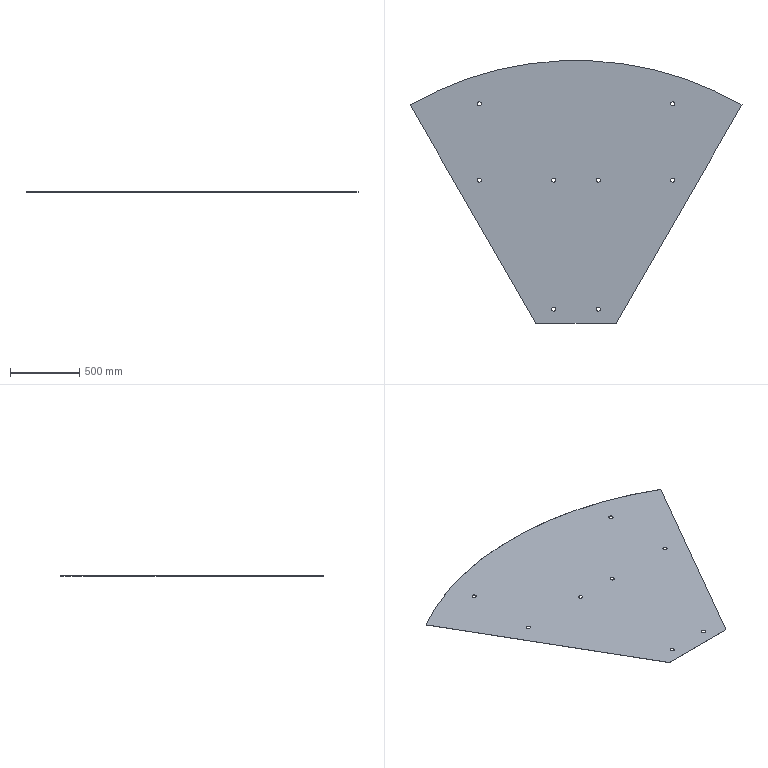Part | SolidWorks | features FlatPattern 1, HoleWzd 1, SMBaseFlange 1, SheetMetal 1 | 1 solid | 22 faces | box 2393 x 1893 x 1 mm | volume 2848544 mm3 | cylinder 17 | plane 5 | commonest cylinder face diameters 30 x16 4786 x1
STEP:
#1=CARTESIAN_POINT('',(-175.,100.,-1.));
#2=VERTEX_POINT('',#1);
#3=CARTESIAN_POINT('',(-145.,100.,-1.));
#4=VERTEX_POINT('',#3);
#5=CARTESIAN_POINT('',(-160.,100.,-1.));
#6=DIRECTION('',(0.,0.,1.));
#7=DIRECTION('',(1.,0.,0.));
#8=AXIS2_PLACEMENT_3D('',#5,#6,#7);
#9=CIRCLE('',#8,15.);
#10=EDGE_CURVE('',#2,#4,#9,.T.);
#11=ORIENTED_EDGE('',*,*,#10,.F.);
#12=CARTESIAN_POINT('',(-175.,100.,0.));
#13=VERTEX_POINT('',#12);
#14=CARTESIAN_POINT('',(-175.,100.,0.));
#15=DIRECTION('',(0.,0.,1.));
#16=VECTOR('',#15,1000.);
#17=LINE('',#14,#16);
#18=EDGE_CURVE('',#2,#13,#17,.T.);
#19=ORIENTED_EDGE('',*,*,#18,.T.);
#20=CARTESIAN_POINT('',(-145.,100.,0.));
#21=VERTEX_POINT('',#20);
#22=CARTESIAN_POINT('',(-160.,100.,0.));
#23=DIRECTION('',(0.,0.,1.));
#24=DIRECTION('',(1.,0.,0.));
#25=AXIS2_PLACEMENT_3D('',#22,#23,#24);
#26=CIRCLE('',#25,15.);
#27=EDGE_CURVE('',#13,#21,#26,.T.);
#28=ORIENTED_EDGE('',*,*,#27,.T.);
#29=CARTESIAN_POINT('',(-145.,100.,0.));
#30=DIRECTION('',(0.,0.,1.));
#31=VECTOR('',#30,1000.);
#32=LINE('',#29,#31);
#33=EDGE_CURVE('',#4,#21,#32,.T.);
#34=ORIENTED_EDGE('',*,*,#33,.F.);
#35=EDGE_LOOP('',(#11,#19,#28,#34));
#36=FACE_OUTER_BOUND('',#35,.T.);
#37=CARTESIAN_POINT('',(-160.,100.,0.));
#38=DIRECTION('',(0.,0.,1.));
#39=DIRECTION('',(1.,0.,0.));
#40=AXIS2_PLACEMENT_3D('',#37,#38,#39);
#41=CYLINDRICAL_SURFACE('',#40,15.);
#42=ADVANCED_FACE('',(#36),#41,.F.);
#43=CARTESIAN_POINT('',(-175.,1031.,-1.));
#44=VERTEX_POINT('',#43);
#45=CARTESIAN_POINT('',(-145.,1031.,-1.));
#46=VERTEX_POINT('',#45);
#47=CARTESIAN_POINT('',(-160.,1031.,-1.));
#48=DIRECTION('',(0.,0.,1.));
#49=DIRECTION('',(1.,0.,0.));
#50=AXIS2_PLACEMENT_3D('',#47,#48,#49);
#51=CIRCLE('',#50,15.);
#52=EDGE_CURVE('',#44,#46,#51,.T.);
#53=ORIENTED_EDGE('',*,*,#52,.F.);
#54=CARTESIAN_POINT('',(-175.,1031.,0.));
#55=VERTEX_POINT('',#54);
#56=CARTESIAN_POINT('',(-175.,1031.,0.));
#57=DIRECTION('',(0.,0.,1.));
#58=VECTOR('',#57,1000.);
#59=LINE('',#56,#58);
#60=EDGE_CURVE('',#44,#55,#59,.T.);
#61=ORIENTED_EDGE('',*,*,#60,.T.);
#62=CARTESIAN_POINT('',(-145.,1031.,0.));
#63=VERTEX_POINT('',#62);
#64=CARTESIAN_POINT('',(-160.,1031.,0.));
#65=DIRECTION('',(0.,0.,1.));
#66=DIRECTION('',(1.,0.,0.));
#67=AXIS2_PLACEMENT_3D('',#64,#65,#66);
#68=CIRCLE('',#67,15.);
#69=EDGE_CURVE('',#55,#63,#68,.T.);
#70=ORIENTED_EDGE('',*,*,#69,.T.);
#71=CARTESIAN_POINT('',(-145.,1031.,0.));
#72=DIRECTION('',(0.,0.,1.));
#73=VECTOR('',#72,1000.);
#74=LINE('',#71,#73);
#75=EDGE_CURVE('',#46,#63,#74,.T.);
#76=ORIENTED_EDGE('',*,*,#75,.F.);
#77=EDGE_LOOP('',(#53,#61,#70,#76));
#78=FACE_OUTER_BOUND('',#77,.T.);
#79=CARTESIAN_POINT('',(-160.,1031.,0.));
#80=DIRECTION('',(0.,0.,1.));
#81=DIRECTION('',(1.,0.,0.));
#82=AXIS2_PLACEMENT_3D('',#79,#80,#81);
#83=CYLINDRICAL_SURFACE('',#82,15.);
#84=ADVANCED_FACE('',(#78),#83,.F.);
#85=CARTESIAN_POINT('',(-712.5,1031.,-1.));
#86=VERTEX_POINT('',#85);
#87=CARTESIAN_POINT('',(-682.5,1031.,-1.));
#88=VERTEX_POINT('',#87);
#89=CARTESIAN_POINT('',(-697.5,1031.,-1.));
#90=DIRECTION('',(0.,0.,1.));
#91=DIRECTION('',(1.,0.,0.));
#92=AXIS2_PLACEMENT_3D('',#89,#90,#91);
#93=CIRCLE('',#92,15.);
#94=EDGE_CURVE('',#86,#88,#93,.T.);
#95=ORIENTED_EDGE('',*,*,#94,.F.);
#96=CARTESIAN_POINT('',(-712.5,1031.,0.));
#97=VERTEX_POINT('',#96);
#98=CARTESIAN_POINT('',(-712.5,1031.,0.));
#99=DIRECTION('',(0.,0.,1.));
#100=VECTOR('',#99,1000.);
#101=LINE('',#98,#100);
#102=EDGE_CURVE('',#86,#97,#101,.T.);
#103=ORIENTED_EDGE('',*,*,#102,.T.);
#104=CARTESIAN_POINT('',(-682.5,1031.,0.));
#105=VERTEX_POINT('',#104);
#106=CARTESIAN_POINT('',(-697.5,1031.,0.));
#107=DIRECTION('',(0.,0.,1.));
#108=DIRECTION('',(1.,0.,0.));
#109=AXIS2_PLACEMENT_3D('',#106,#107,#108);
#110=CIRCLE('',#109,15.);
#111=EDGE_CURVE('',#97,#105,#110,.T.);
#112=ORIENTED_EDGE('',*,*,#111,.T.);
#113=CARTESIAN_POINT('',(-682.5,1031.,0.));
#114=DIRECTION('',(0.,0.,1.));
#115=VECTOR('',#114,1000.);
#116=LINE('',#113,#115);
#117=EDGE_CURVE('',#88,#105,#116,.T.);
#118=ORIENTED_EDGE('',*,*,#117,.F.);
#119=EDGE_LOOP('',(#95,#103,#112,#118));
#120=FACE_OUTER_BOUND('',#119,.T.);
#121=CARTESIAN_POINT('',(-697.5,1031.,0.));
#122=DIRECTION('',(0.,0.,1.));
#123=DIRECTION('',(1.,0.,0.));
#124=AXIS2_PLACEMENT_3D('',#121,#122,#123);
#125=CYLINDRICAL_SURFACE('',#124,15.);
#126=ADVANCED_FACE('',(#120),#125,.F.);
#127=CARTESIAN_POINT('',(-712.5,1581.,-1.));
#128=VERTEX_POINT('',#127);
#129=CARTESIAN_POINT('',(-682.5,1581.,-1.));
#130=VERTEX_POINT('',#129);
#131=CARTESIAN_POINT('',(-697.5,1581.,-1.));
#132=DIRECTION('',(0.,0.,1.));
#133=DIRECTION('',(1.,0.,0.));
#134=AXIS2_PLACEMENT_3D('',#131,#132,#133);
#135=CIRCLE('',#134,15.);
#136=EDGE_CURVE('',#128,#130,#135,.T.);
#137=ORIENTED_EDGE('',*,*,#136,.F.);
#138=CARTESIAN_POINT('',(-712.5,1581.,0.));
#139=VERTEX_POINT('',#138);
#140=CARTESIAN_POINT('',(-712.5,1581.,0.));
#141=DIRECTION('',(0.,0.,1.));
#142=VECTOR('',#141,1000.);
#143=LINE('',#140,#142);
#144=EDGE_CURVE('',#128,#139,#143,.T.);
#145=ORIENTED_EDGE('',*,*,#144,.T.);
#146=CARTESIAN_POINT('',(-682.5,1581.,0.));
#147=VERTEX_POINT('',#146);
#148=CARTESIAN_POINT('',(-697.5,1581.,0.));
#149=DIRECTION('',(0.,0.,1.));
#150=DIRECTION('',(1.,0.,0.));
#151=AXIS2_PLACEMENT_3D('',#148,#149,#150);
#152=CIRCLE('',#151,15.);
#153=EDGE_CURVE('',#139,#147,#152,.T.);
#154=ORIENTED_EDGE('',*,*,#153,.T.);
#155=CARTESIAN_POINT('',(-682.5,1581.,0.));
#156=DIRECTION('',(0.,0.,1.));
#157=VECTOR('',#156,1000.);
#158=LINE('',#155,#157);
#159=EDGE_CURVE('',#130,#147,#158,.T.);
#160=ORIENTED_EDGE('',*,*,#159,.F.);
#161=EDGE_LOOP('',(#137,#145,#154,#160));
#162=FACE_OUTER_BOUND('',#161,.T.);
#163=CARTESIAN_POINT('',(-697.5,1581.,0.));
#164=DIRECTION('',(0.,0.,1.));
#165=DIRECTION('',(1.,0.,0.));
#166=AXIS2_PLACEMENT_3D('',#163,#164,#165);
#167=CYLINDRICAL_SURFACE('',#166,15.);
#168=ADVANCED_FACE('',(#162),#167,.F.);
#169=CARTESIAN_POINT('',(682.5,1581.,-1.));
#170=VERTEX_POINT('',#169);
#171=CARTESIAN_POINT('',(712.5,1581.,-1.));
#172=VERTEX_POINT('',#171);
#173=CARTESIAN_POINT('',(697.5,1581.,-1.));
#174=DIRECTION('',(0.,0.,1.));
#175=DIRECTION('',(1.,0.,0.));
#176=AXIS2_PLACEMENT_3D('',#173,#174,#175);
#177=CIRCLE('',#176,15.);
#178=EDGE_CURVE('',#170,#172,#177,.T.);
#179=ORIENTED_EDGE('',*,*,#178,.F.);
#180=CARTESIAN_POINT('',(682.5,1581.,0.));
#181=VERTEX_POINT('',#180);
#182=CARTESIAN_POINT('',(682.5,1581.,0.));
#183=DIRECTION('',(0.,0.,1.));
#184=VECTOR('',#183,1000.);
#185=LINE('',#182,#184);
#186=EDGE_CURVE('',#170,#181,#185,.T.);
#187=ORIENTED_EDGE('',*,*,#186,.T.);
#188=CARTESIAN_POINT('',(712.5,1581.,0.));
#189=VERTEX_POINT('',#188);
#190=CARTESIAN_POINT('',(697.5,1581.,0.));
#191=DIRECTION('',(0.,0.,1.));
#192=DIRECTION('',(1.,0.,0.));
#193=AXIS2_PLACEMENT_3D('',#190,#191,#192);
#194=CIRCLE('',#193,15.);
#195=EDGE_CURVE('',#181,#189,#194,.T.);
#196=ORIENTED_EDGE('',*,*,#195,.T.);
#197=CARTESIAN_POINT('',(712.5,1581.,0.));
#198=DIRECTION('',(0.,0.,1.));
#199=VECTOR('',#198,1000.);
#200=LINE('',#197,#199);
#201=EDGE_CURVE('',#172,#189,#200,.T.);
#202=ORIENTED_EDGE('',*,*,#201,.F.);
#203=EDGE_LOOP('',(#179,#187,#196,#202));
#204=FACE_OUTER_BOUND('',#203,.T.);
#205=CARTESIAN_POINT('',(697.5,1581.,0.));
#206=DIRECTION('',(0.,0.,1.));
#207=DIRECTION('',(1.,0.,0.));
#208=AXIS2_PLACEMENT_3D('',#205,#206,#207);
#209=CYLINDRICAL_SURFACE('',#208,15.);
#210=ADVANCED_FACE('',(#204),#209,.F.);
#211=CARTESIAN_POINT('',(682.5,1031.,-1.));
#212=VERTEX_POINT('',#211);
#213=CARTESIAN_POINT('',(712.5,1031.,-1.));
#214=VERTEX_POINT('',#213);
#215=CARTESIAN_POINT('',(697.5,1031.,-1.));
#216=DIRECTION('',(0.,0.,1.));
#217=DIRECTION('',(1.,0.,0.));
#218=AXIS2_PLACEMENT_3D('',#215,#216,#217);
#219=CIRCLE('',#218,15.);
#220=EDGE_CURVE('',#212,#214,#219,.T.);
#221=ORIENTED_EDGE('',*,*,#220,.F.);
#222=CARTESIAN_POINT('',(682.5,1031.,0.));
#223=VERTEX_POINT('',#222);
#224=CARTESIAN_POINT('',(682.5,1031.,0.));
#225=DIRECTION('',(0.,0.,1.));
#226=VECTOR('',#225,1000.);
#227=LINE('',#224,#226);
#228=EDGE_CURVE('',#212,#223,#227,.T.);
#229=ORIENTED_EDGE('',*,*,#228,.T.);
#230=CARTESIAN_POINT('',(712.5,1031.,0.));
#231=VERTEX_POINT('',#230);
#232=CARTESIAN_POINT('',(697.5,1031.,0.));
#233=DIRECTION('',(0.,0.,1.));
#234=DIRECTION('',(1.,0.,0.));
#235=AXIS2_PLACEMENT_3D('',#232,#233,#234);
#236=CIRCLE('',#235,15.);
#237=EDGE_CURVE('',#223,#231,#236,.T.);
#238=ORIENTED_EDGE('',*,*,#237,.T.);
#239=CARTESIAN_POINT('',(712.5,1031.,0.));
#240=DIRECTION('',(0.,0.,1.));
#241=VECTOR('',#240,1000.);
#242=LINE('',#239,#241);
#243=EDGE_CURVE('',#214,#231,#242,.T.);
#244=ORIENTED_EDGE('',*,*,#243,.F.);
#245=EDGE_LOOP('',(#221,#229,#238,#244));
#246=FACE_OUTER_BOUND('',#245,.T.);
#247=CARTESIAN_POINT('',(697.5,1031.,0.));
#248=DIRECTION('',(0.,0.,1.));
#249=DIRECTION('',(1.,0.,0.));
#250=AXIS2_PLACEMENT_3D('',#247,#248,#249);
#251=CYLINDRICAL_SURFACE('',#250,15.);
#252=ADVANCED_FACE('',(#246),#251,.F.);
#253=CARTESIAN_POINT('',(145.,1031.,-1.));
#254=VERTEX_POINT('',#253);
#255=CARTESIAN_POINT('',(175.,1031.,-1.));
#256=VERTEX_POINT('',#255);
#257=CARTESIAN_POINT('',(160.,1031.,-1.));
#258=DIRECTION('',(0.,0.,1.));
#259=DIRECTION('',(1.,0.,0.));
#260=AXIS2_PLACEMENT_3D('',#257,#258,#259);
#261=CIRCLE('',#260,15.);
#262=EDGE_CURVE('',#254,#256,#261,.T.);
#263=ORIENTED_EDGE('',*,*,#262,.F.);
#264=CARTESIAN_POINT('',(145.,1031.,0.));
#265=VERTEX_POINT('',#264);
#266=CARTESIAN_POINT('',(145.,1031.,0.));
#267=DIRECTION('',(0.,0.,1.));
#268=VECTOR('',#267,1000.);
#269=LINE('',#266,#268);
#270=EDGE_CURVE('',#254,#265,#269,.T.);
#271=ORIENTED_EDGE('',*,*,#270,.T.);
#272=CARTESIAN_POINT('',(175.,1031.,0.));
#273=VERTEX_POINT('',#272);
#274=CARTESIAN_POINT('',(160.,1031.,0.));
#275=DIRECTION('',(0.,0.,1.));
#276=DIRECTION('',(1.,0.,0.));
#277=AXIS2_PLACEMENT_3D('',#274,#275,#276);
#278=CIRCLE('',#277,15.);
#279=EDGE_CURVE('',#265,#273,#278,.T.);
#280=ORIENTED_EDGE('',*,*,#279,.T.);
#281=CARTESIAN_POINT('',(175.,1031.,0.));
#282=DIRECTION('',(0.,0.,1.));
#283=VECTOR('',#282,1000.);
#284=LINE('',#281,#283);
#285=EDGE_CURVE('',#256,#273,#284,.T.);
#286=ORIENTED_EDGE('',*,*,#285,.F.);
#287=EDGE_LOOP('',(#263,#271,#280,#286));
#288=FACE_OUTER_BOUND('',#287,.T.);
#289=CARTESIAN_POINT('',(160.,1031.,0.));
#290=DIRECTION('',(0.,0.,1.));
#291=DIRECTION('',(1.,0.,0.));
#292=AXIS2_PLACEMENT_3D('',#289,#290,#291);
#293=CYLINDRICAL_SURFACE('',#292,15.);
#294=ADVANCED_FACE('',(#288),#293,.F.);
#295=CARTESIAN_POINT('',(145.,100.,-1.));
#296=VERTEX_POINT('',#295);
#297=CARTESIAN_POINT('',(175.,100.,-1.));
#298=VERTEX_POINT('',#297);
#299=CARTESIAN_POINT('',(160.,100.,-1.));
#300=DIRECTION('',(0.,0.,1.));
#301=DIRECTION('',(1.,0.,0.));
#302=AXIS2_PLACEMENT_3D('',#299,#300,#301);
#303=CIRCLE('',#302,15.);
#304=EDGE_CURVE('',#296,#298,#303,.T.);
#305=ORIENTED_EDGE('',*,*,#304,.F.);
#306=CARTESIAN_POINT('',(145.,100.,0.));
#307=VERTEX_POINT('',#306);
#308=CARTESIAN_POINT('',(145.,100.,0.));
#309=DIRECTION('',(0.,0.,1.));
#310=VECTOR('',#309,1000.);
#311=LINE('',#308,#310);
#312=EDGE_CURVE('',#296,#307,#311,.T.);
#313=ORIENTED_EDGE('',*,*,#312,.T.);
#314=CARTESIAN_POINT('',(175.,100.,0.));
#315=VERTEX_POINT('',#314);
#316=CARTESIAN_POINT('',(160.,100.,0.));
#317=DIRECTION('',(0.,0.,1.));
#318=DIRECTION('',(1.,0.,0.));
#319=AXIS2_PLACEMENT_3D('',#316,#317,#318);
#320=CIRCLE('',#319,15.);
#321=EDGE_CURVE('',#307,#315,#320,.T.);
#322=ORIENTED_EDGE('',*,*,#321,.T.);
#323=CARTESIAN_POINT('',(175.,100.,0.));
#324=DIRECTION('',(0.,0.,1.));
#325=VECTOR('',#324,1000.);
#326=LINE('',#323,#325);
#327=EDGE_CURVE('',#298,#315,#326,.T.);
#328=ORIENTED_EDGE('',*,*,#327,.F.);
#329=EDGE_LOOP('',(#305,#313,#322,#328));
#330=FACE_OUTER_BOUND('',#329,.T.);
#331=CARTESIAN_POINT('',(160.,100.,0.));
#332=DIRECTION('',(0.,0.,1.));
#333=DIRECTION('',(1.,0.,0.));
#334=AXIS2_PLACEMENT_3D('',#331,#332,#333);
#335=CYLINDRICAL_SURFACE('',#334,15.);
#336=ADVANCED_FACE('',(#330),#335,.F.);
#337=CARTESIAN_POINT('',(288.5,0.,0.));
#338=VERTEX_POINT('',#337);
#339=CARTESIAN_POINT('',(1196.5,1572.702,0.));
#340=VERTEX_POINT('',#339);
#341=CARTESIAN_POINT('',(288.5,0.,0.));
#342=DIRECTION('',(0.5,0.866,0.));
#343=VECTOR('',#342,1000.);
#344=LINE('',#341,#343);
#345=EDGE_CURVE('',#338,#340,#344,.T.);
#346=ORIENTED_EDGE('',*,*,#345,.F.);
#347=CARTESIAN_POINT('',(288.5,0.,-1.));
#348=VERTEX_POINT('',#347);
#349=CARTESIAN_POINT('',(288.5,0.,-1.));
#350=DIRECTION('',(0.,0.,1.));
#351=VECTOR('',#350,1000.);
#352=LINE('',#349,#351);
#353=EDGE_CURVE('',#348,#338,#352,.T.);
#354=ORIENTED_EDGE('',*,*,#353,.F.);
#355=CARTESIAN_POINT('',(1196.5,1572.702,-1.));
#356=VERTEX_POINT('',#355);
#357=CARTESIAN_POINT('',(288.5,0.,-1.));
#358=DIRECTION('',(0.5,0.866,0.));
#359=VECTOR('',#358,1000.);
#360=LINE('',#357,#359);
#361=EDGE_CURVE('',#348,#356,#360,.T.);
#362=ORIENTED_EDGE('',*,*,#361,.T.);
#363=CARTESIAN_POINT('',(1196.5,1572.702,-1.));
#364=DIRECTION('',(0.,0.,1.));
#365=VECTOR('',#364,1000.);
#366=LINE('',#363,#365);
#367=EDGE_CURVE('',#356,#340,#366,.T.);
#368=ORIENTED_EDGE('',*,*,#367,.T.);
#369=EDGE_LOOP('',(#346,#354,#362,#368));
#370=FACE_OUTER_BOUND('',#369,.T.);
#371=CARTESIAN_POINT('',(288.5,0.,-1.));
#372=DIRECTION('',(0.866,-0.5,0.));
#373=DIRECTION('',(0.5,0.866,0.));
#374=AXIS2_PLACEMENT_3D('',#371,#372,#373);
#375=PLANE('',#374);
#376=ADVANCED_FACE('',(#370),#375,.T.);
#377=CARTESIAN_POINT('',(-288.5,0.,0.));
#378=VERTEX_POINT('',#377);
#379=CARTESIAN_POINT('',(-288.5,0.,0.));
#380=DIRECTION('',(1.,0.,0.));
#381=VECTOR('',#380,1000.);
#382=LINE('',#379,#381);
#383=EDGE_CURVE('',#378,#338,#382,.T.);
#384=ORIENTED_EDGE('',*,*,#383,.F.);
#385=CARTESIAN_POINT('',(-288.5,0.,-1.));
#386=VERTEX_POINT('',#385);
#387=CARTESIAN_POINT('',(-288.5,0.,-1.));
#388=DIRECTION('',(0.,0.,1.));
#389=VECTOR('',#388,1000.);
#390=LINE('',#387,#389);
#391=EDGE_CURVE('',#386,#378,#390,.T.);
#392=ORIENTED_EDGE('',*,*,#391,.F.);
#393=CARTESIAN_POINT('',(-288.5,0.,-1.));
#394=DIRECTION('',(1.,0.,0.));
#395=VECTOR('',#394,1000.);
#396=LINE('',#393,#395);
#397=EDGE_CURVE('',#386,#348,#396,.T.);
#398=ORIENTED_EDGE('',*,*,#397,.T.);
#399=ORIENTED_EDGE('',*,*,#353,.T.);
#400=EDGE_LOOP('',(#384,#392,#398,#399));
#401=FACE_OUTER_BOUND('',#400,.T.);
#402=CARTESIAN_POINT('',(-288.5,0.,-1.));
#403=DIRECTION('',(0.,-1.,0.));
#404=DIRECTION('',(0.,0.,-1.));
#405=AXIS2_PLACEMENT_3D('',#402,#403,#404);
#406=PLANE('',#405);
#407=ADVANCED_FACE('',(#401),#406,.T.);
#408=CARTESIAN_POINT('',(-1196.5,1572.702,0.));
#409=VERTEX_POINT('',#408);
#410=CARTESIAN_POINT('',(-288.5,0.,0.));
#411=DIRECTION('',(0.5,-0.866,0.));
#412=VECTOR('',#411,1000.);
#413=LINE('',#410,#412);
#414=EDGE_CURVE('',#409,#378,#413,.T.);
#415=ORIENTED_EDGE('',*,*,#414,.F.);
#416=CARTESIAN_POINT('',(-1196.5,1572.702,-1.));
#417=VERTEX_POINT('',#416);
#418=CARTESIAN_POINT('',(-1196.5,1572.702,-1.));
#419=DIRECTION('',(0.,0.,1.));
#420=VECTOR('',#419,1000.);
#421=LINE('',#418,#420);
#422=EDGE_CURVE('',#417,#409,#421,.T.);
#423=ORIENTED_EDGE('',*,*,#422,.F.);
#424=CARTESIAN_POINT('',(-288.5,0.,-1.));
#425=DIRECTION('',(0.5,-0.866,0.));
#426=VECTOR('',#425,1000.);
#427=LINE('',#424,#426);
#428=EDGE_CURVE('',#417,#386,#427,.T.);
#429=ORIENTED_EDGE('',*,*,#428,.T.);
#430=ORIENTED_EDGE('',*,*,#391,.T.);
#431=EDGE_LOOP('',(#415,#423,#429,#430));
#432=FACE_OUTER_BOUND('',#431,.T.);
#433=CARTESIAN_POINT('',(-288.5,0.,-1.));
#434=DIRECTION('',(-0.866,-0.5,0.));
#435=DIRECTION('',(0.5,-0.866,0.));
#436=AXIS2_PLACEMENT_3D('',#433,#434,#435);
#437=PLANE('',#436);
#438=ADVANCED_FACE('',(#432),#437,.T.);
#439=CARTESIAN_POINT('',(0.,-499.697,0.));
#440=DIRECTION('',(0.,0.,1.));
#441=DIRECTION('',(1.,0.,0.));
#442=AXIS2_PLACEMENT_3D('',#439,#440,#441);
#443=CIRCLE('',#442,2393.);
#444=EDGE_CURVE('',#340,#409,#443,.T.);
#445=ORIENTED_EDGE('',*,*,#444,.F.);
#446=ORIENTED_EDGE('',*,*,#367,.F.);
#447=CARTESIAN_POINT('',(0.,-499.697,-1.));
#448=DIRECTION('',(0.,0.,1.));
#449=DIRECTION('',(1.,0.,0.));
#450=AXIS2_PLACEMENT_3D('',#447,#448,#449);
#451=CIRCLE('',#450,2393.);
#452=EDGE_CURVE('',#356,#417,#451,.T.);
#453=ORIENTED_EDGE('',*,*,#452,.T.);
#454=ORIENTED_EDGE('',*,*,#422,.T.);
#455=EDGE_LOOP('',(#445,#446,#453,#454));
#456=FACE_OUTER_BOUND('',#455,.T.);
#457=CARTESIAN_POINT('',(0.,-499.697,-1.));
#458=DIRECTION('',(0.,0.,1.));
#459=DIRECTION('',(1.,0.,0.));
#460=AXIS2_PLACEMENT_3D('',#457,#458,#459);
#461=CYLINDRICAL_SURFACE('',#460,2393.);
#462=ADVANCED_FACE('',(#456),#461,.T.);
#463=CARTESIAN_POINT('',(-160.,100.,-1.));
#464=DIRECTION('',(0.,0.,1.));
#465=DIRECTION('',(1.,0.,0.));
#466=AXIS2_PLACEMENT_3D('',#463,#464,#465);
#467=CIRCLE('',#466,15.);
#468=EDGE_CURVE('',#4,#2,#467,.T.);
#469=ORIENTED_EDGE('',*,*,#468,.T.);
#470=ORIENTED_EDGE('',*,*,#10,.T.);
#471=EDGE_LOOP('',(#469,#470));
#472=FACE_BOUND('',#471,.T.);
#473=CARTESIAN_POINT('',(-160.,1031.,-1.));
#474=DIRECTION('',(0.,0.,1.));
#475=DIRECTION('',(1.,0.,0.));
#476=AXIS2_PLACEMENT_3D('',#473,#474,#475);
#477=CIRCLE('',#476,15.);
#478=EDGE_CURVE('',#46,#44,#477,.T.);
#479=ORIENTED_EDGE('',*,*,#478,.T.);
#480=ORIENTED_EDGE('',*,*,#52,.T.);
#481=EDGE_LOOP('',(#479,#480));
#482=FACE_BOUND('',#481,.T.);
#483=CARTESIAN_POINT('',(-697.5,1031.,-1.));
#484=DIRECTION('',(0.,0.,1.));
#485=DIRECTION('',(1.,0.,0.));
#486=AXIS2_PLACEMENT_3D('',#483,#484,#485);
#487=CIRCLE('',#486,15.);
#488=EDGE_CURVE('',#88,#86,#487,.T.);
#489=ORIENTED_EDGE('',*,*,#488,.T.);
#490=ORIENTED_EDGE('',*,*,#94,.T.);
#491=EDGE_LOOP('',(#489,#490));
#492=FACE_BOUND('',#491,.T.);
#493=CARTESIAN_POINT('',(-697.5,1581.,-1.));
#494=DIRECTION('',(0.,0.,1.));
#495=DIRECTION('',(1.,0.,0.));
#496=AXIS2_PLACEMENT_3D('',#493,#494,#495);
#497=CIRCLE('',#496,15.);
#498=EDGE_CURVE('',#130,#128,#497,.T.);
#499=ORIENTED_EDGE('',*,*,#498,.T.);
#500=ORIENTED_EDGE('',*,*,#136,.T.);
#501=EDGE_LOOP('',(#499,#500));
#502=FACE_BOUND('',#501,.T.);
#503=CARTESIAN_POINT('',(697.5,1581.,-1.));
#504=DIRECTION('',(0.,0.,1.));
#505=DIRECTION('',(1.,0.,0.));
#506=AXIS2_PLACEMENT_3D('',#503,#504,#505);
#507=CIRCLE('',#506,15.);
#508=EDGE_CURVE('',#172,#170,#507,.T.);
#509=ORIENTED_EDGE('',*,*,#508,.T.);
#510=ORIENTED_EDGE('',*,*,#178,.T.);
#511=EDGE_LOOP('',(#509,#510));
#512=FACE_BOUND('',#511,.T.);
#513=CARTESIAN_POINT('',(697.5,1031.,-1.));
#514=DIRECTION('',(0.,0.,1.));
#515=DIRECTION('',(1.,0.,0.));
#516=AXIS2_PLACEMENT_3D('',#513,#514,#515);
#517=CIRCLE('',#516,15.);
#518=EDGE_CURVE('',#214,#212,#517,.T.);
#519=ORIENTED_EDGE('',*,*,#518,.T.);
#520=ORIENTED_EDGE('',*,*,#220,.T.);
#521=EDGE_LOOP('',(#519,#520));
#522=FACE_BOUND('',#521,.T.);
#523=CARTESIAN_POINT('',(160.,1031.,-1.));
#524=DIRECTION('',(0.,0.,1.));
#525=DIRECTION('',(1.,0.,0.));
#526=AXIS2_PLACEMENT_3D('',#523,#524,#525);
#527=CIRCLE('',#526,15.);
#528=EDGE_CURVE('',#256,#254,#527,.T.);
#529=ORIENTED_EDGE('',*,*,#528,.T.);
#530=ORIENTED_EDGE('',*,*,#262,.T.);
#531=EDGE_LOOP('',(#529,#530));
#532=FACE_BOUND('',#531,.T.);
#533=CARTESIAN_POINT('',(160.,100.,-1.));
#534=DIRECTION('',(0.,0.,1.));
#535=DIRECTION('',(1.,0.,0.));
#536=AXIS2_PLACEMENT_3D('',#533,#534,#535);
#537=CIRCLE('',#536,15.);
#538=EDGE_CURVE('',#298,#296,#537,.T.);
#539=ORIENTED_EDGE('',*,*,#538,.T.);
#540=ORIENTED_EDGE('',*,*,#304,.T.);
#541=EDGE_LOOP('',(#539,#540));
#542=FACE_BOUND('',#541,.T.);
#543=ORIENTED_EDGE('',*,*,#361,.F.);
#544=ORIENTED_EDGE('',*,*,#397,.F.);
#545=ORIENTED_EDGE('',*,*,#428,.F.);
#546=ORIENTED_EDGE('',*,*,#452,.F.);
#547=EDGE_LOOP('',(#543,#544,#545,#546));
#548=FACE_OUTER_BOUND('',#547,.T.);
#549=CARTESIAN_POINT('',(0.,-499.697,-1.));
#550=DIRECTION('',(0.,0.,1.));
#551=DIRECTION('',(1.,0.,0.));
#552=AXIS2_PLACEMENT_3D('',#549,#550,#551);
#553=PLANE('',#552);
#554=ADVANCED_FACE('',(#472,#482,#492,#502,#512,#522,#532,#542,#548),#553,.F.);
#555=CARTESIAN_POINT('',(-160.,100.,0.));
#556=DIRECTION('',(0.,0.,1.));
#557=DIRECTION('',(1.,0.,0.));
#558=AXIS2_PLACEMENT_3D('',#555,#556,#557);
#559=CIRCLE('',#558,15.);
#560=EDGE_CURVE('',#21,#13,#559,.T.);
#561=ORIENTED_EDGE('',*,*,#560,.F.);
#562=ORIENTED_EDGE('',*,*,#27,.F.);
#563=EDGE_LOOP('',(#561,#562));
#564=FACE_BOUND('',#563,.T.);
#565=CARTESIAN_POINT('',(-160.,1031.,0.));
#566=DIRECTION('',(0.,0.,1.));
#567=DIRECTION('',(1.,0.,0.));
#568=AXIS2_PLACEMENT_3D('',#565,#566,#567);
#569=CIRCLE('',#568,15.);
#570=EDGE_CURVE('',#63,#55,#569,.T.);
#571=ORIENTED_EDGE('',*,*,#570,.F.);
#572=ORIENTED_EDGE('',*,*,#69,.F.);
#573=EDGE_LOOP('',(#571,#572));
#574=FACE_BOUND('',#573,.T.);
#575=CARTESIAN_POINT('',(-697.5,1031.,0.));
#576=DIRECTION('',(0.,0.,1.));
#577=DIRECTION('',(1.,0.,0.));
#578=AXIS2_PLACEMENT_3D('',#575,#576,#577);
#579=CIRCLE('',#578,15.);
#580=EDGE_CURVE('',#105,#97,#579,.T.);
#581=ORIENTED_EDGE('',*,*,#580,.F.);
#582=ORIENTED_EDGE('',*,*,#111,.F.);
#583=EDGE_LOOP('',(#581,#582));
#584=FACE_BOUND('',#583,.T.);
#585=CARTESIAN_POINT('',(-697.5,1581.,0.));
#586=DIRECTION('',(0.,0.,1.));
#587=DIRECTION('',(1.,0.,0.));
#588=AXIS2_PLACEMENT_3D('',#585,#586,#587);
#589=CIRCLE('',#588,15.);
#590=EDGE_CURVE('',#147,#139,#589,.T.);
#591=ORIENTED_EDGE('',*,*,#590,.F.);
#592=ORIENTED_EDGE('',*,*,#153,.F.);
#593=EDGE_LOOP('',(#591,#592));
#594=FACE_BOUND('',#593,.T.);
#595=CARTESIAN_POINT('',(697.5,1581.,0.));
#596=DIRECTION('',(0.,0.,1.));
#597=DIRECTION('',(1.,0.,0.));
#598=AXIS2_PLACEMENT_3D('',#595,#596,#597);
#599=CIRCLE('',#598,15.);
#600=EDGE_CURVE('',#189,#181,#599,.T.);
#601=ORIENTED_EDGE('',*,*,#600,.F.);
#602=ORIENTED_EDGE('',*,*,#195,.F.);
#603=EDGE_LOOP('',(#601,#602));
#604=FACE_BOUND('',#603,.T.);
#605=CARTESIAN_POINT('',(697.5,1031.,0.));
#606=DIRECTION('',(0.,0.,1.));
#607=DIRECTION('',(1.,0.,0.));
#608=AXIS2_PLACEMENT_3D('',#605,#606,#607);
#609=CIRCLE('',#608,15.);
#610=EDGE_CURVE('',#231,#223,#609,.T.);
#611=ORIENTED_EDGE('',*,*,#610,.F.);
#612=ORIENTED_EDGE('',*,*,#237,.F.);
#613=EDGE_LOOP('',(#611,#612));
#614=FACE_BOUND('',#613,.T.);
#615=CARTESIAN_POINT('',(160.,1031.,0.));
#616=DIRECTION('',(0.,0.,1.));
#617=DIRECTION('',(1.,0.,0.));
#618=AXIS2_PLACEMENT_3D('',#615,#616,#617);
#619=CIRCLE('',#618,15.);
#620=EDGE_CURVE('',#273,#265,#619,.T.);
#621=ORIENTED_EDGE('',*,*,#620,.F.);
#622=ORIENTED_EDGE('',*,*,#279,.F.);
#623=EDGE_LOOP('',(#621,#622));
#624=FACE_BOUND('',#623,.T.);
#625=CARTESIAN_POINT('',(160.,100.,0.));
#626=DIRECTION('',(0.,0.,1.));
#627=DIRECTION('',(1.,0.,0.));
#628=AXIS2_PLACEMENT_3D('',#625,#626,#627);
#629=CIRCLE('',#628,15.);
#630=EDGE_CURVE('',#315,#307,#629,.T.);
#631=ORIENTED_EDGE('',*,*,#630,.F.);
#632=ORIENTED_EDGE('',*,*,#321,.F.);
#633=EDGE_LOOP('',(#631,#632));
#634=FACE_BOUND('',#633,.T.);
#635=ORIENTED_EDGE('',*,*,#345,.T.);
#636=ORIENTED_EDGE('',*,*,#444,.T.);
#637=ORIENTED_EDGE('',*,*,#414,.T.);
#638=ORIENTED_EDGE('',*,*,#383,.T.);
#639=EDGE_LOOP('',(#635,#636,#637,#638));
#640=FACE_OUTER_BOUND('',#639,.T.);
#641=CARTESIAN_POINT('',(0.,-499.697,0.));
#642=DIRECTION('',(0.,0.,1.));
#643=DIRECTION('',(1.,0.,0.));
#644=AXIS2_PLACEMENT_3D('',#641,#642,#643);
#645=PLANE('',#644);
#646=ADVANCED_FACE('',(#564,#574,#584,#594,#604,#614,#624,#634,#640),#645,.T.);
#647=ORIENTED_EDGE('',*,*,#312,.F.);
#648=ORIENTED_EDGE('',*,*,#538,.F.);
#649=ORIENTED_EDGE('',*,*,#327,.T.);
#650=ORIENTED_EDGE('',*,*,#630,.T.);
#651=EDGE_LOOP('',(#647,#648,#649,#650));
#652=FACE_OUTER_BOUND('',#651,.T.);
#653=CARTESIAN_POINT('',(160.,100.,0.));
#654=DIRECTION('',(0.,0.,1.));
#655=DIRECTION('',(1.,0.,0.));
#656=AXIS2_PLACEMENT_3D('',#653,#654,#655);
#657=CYLINDRICAL_SURFACE('',#656,15.);
#658=ADVANCED_FACE('',(#652),#657,.F.);
#659=ORIENTED_EDGE('',*,*,#270,.F.);
#660=ORIENTED_EDGE('',*,*,#528,.F.);
#661=ORIENTED_EDGE('',*,*,#285,.T.);
#662=ORIENTED_EDGE('',*,*,#620,.T.);
#663=EDGE_LOOP('',(#659,#660,#661,#662));
#664=FACE_OUTER_BOUND('',#663,.T.);
#665=CARTESIAN_POINT('',(160.,1031.,0.));
#666=DIRECTION('',(0.,0.,1.));
#667=DIRECTION('',(1.,0.,0.));
#668=AXIS2_PLACEMENT_3D('',#665,#666,#667);
#669=CYLINDRICAL_SURFACE('',#668,15.);
#670=ADVANCED_FACE('',(#664),#669,.F.);
#671=ORIENTED_EDGE('',*,*,#228,.F.);
#672=ORIENTED_EDGE('',*,*,#518,.F.);
#673=ORIENTED_EDGE('',*,*,#243,.T.);
#674=ORIENTED_EDGE('',*,*,#610,.T.);
#675=EDGE_LOOP('',(#671,#672,#673,#674));
#676=FACE_OUTER_BOUND('',#675,.T.);
#677=CARTESIAN_POINT('',(697.5,1031.,0.));
#678=DIRECTION('',(0.,0.,1.));
#679=DIRECTION('',(1.,0.,0.));
#680=AXIS2_PLACEMENT_3D('',#677,#678,#679);
#681=CYLINDRICAL_SURFACE('',#680,15.);
#682=ADVANCED_FACE('',(#676),#681,.F.);
#683=ORIENTED_EDGE('',*,*,#186,.F.);
#684=ORIENTED_EDGE('',*,*,#508,.F.);
#685=ORIENTED_EDGE('',*,*,#201,.T.);
#686=ORIENTED_EDGE('',*,*,#600,.T.);
#687=EDGE_LOOP('',(#683,#684,#685,#686));
#688=FACE_OUTER_BOUND('',#687,.T.);
#689=CARTESIAN_POINT('',(697.5,1581.,0.));
#690=DIRECTION('',(0.,0.,1.));
#691=DIRECTION('',(1.,0.,0.));
#692=AXIS2_PLACEMENT_3D('',#689,#690,#691);
#693=CYLINDRICAL_SURFACE('',#692,15.);
#694=ADVANCED_FACE('',(#688),#693,.F.);
#695=ORIENTED_EDGE('',*,*,#144,.F.);
#696=ORIENTED_EDGE('',*,*,#498,.F.);
#697=ORIENTED_EDGE('',*,*,#159,.T.);
#698=ORIENTED_EDGE('',*,*,#590,.T.);
#699=EDGE_LOOP('',(#695,#696,#697,#698));
#700=FACE_OUTER_BOUND('',#699,.T.);
#701=CARTESIAN_POINT('',(-697.5,1581.,0.));
#702=DIRECTION('',(0.,0.,1.));
#703=DIRECTION('',(1.,0.,0.));
#704=AXIS2_PLACEMENT_3D('',#701,#702,#703);
#705=CYLINDRICAL_SURFACE('',#704,15.);
#706=ADVANCED_FACE('',(#700),#705,.F.);
#707=ORIENTED_EDGE('',*,*,#102,.F.);
#708=ORIENTED_EDGE('',*,*,#488,.F.);
#709=ORIENTED_EDGE('',*,*,#117,.T.);
#710=ORIENTED_EDGE('',*,*,#580,.T.);
#711=EDGE_LOOP('',(#707,#708,#709,#710));
#712=FACE_OUTER_BOUND('',#711,.T.);
#713=CARTESIAN_POINT('',(-697.5,1031.,0.));
#714=DIRECTION('',(0.,0.,1.));
#715=DIRECTION('',(1.,0.,0.));
#716=AXIS2_PLACEMENT_3D('',#713,#714,#715);
#717=CYLINDRICAL_SURFACE('',#716,15.);
#718=ADVANCED_FACE('',(#712),#717,.F.);
#719=ORIENTED_EDGE('',*,*,#60,.F.);
#720=ORIENTED_EDGE('',*,*,#478,.F.);
#721=ORIENTED_EDGE('',*,*,#75,.T.);
#722=ORIENTED_EDGE('',*,*,#570,.T.);
#723=EDGE_LOOP('',(#719,#720,#721,#722));
#724=FACE_OUTER_BOUND('',#723,.T.);
#725=CARTESIAN_POINT('',(-160.,1031.,0.));
#726=DIRECTION('',(0.,0.,1.));
#727=DIRECTION('',(1.,0.,0.));
#728=AXIS2_PLACEMENT_3D('',#725,#726,#727);
#729=CYLINDRICAL_SURFACE('',#728,15.);
#730=ADVANCED_FACE('',(#724),#729,.F.);
#731=ORIENTED_EDGE('',*,*,#18,.F.);
#732=ORIENTED_EDGE('',*,*,#468,.F.);
#733=ORIENTED_EDGE('',*,*,#33,.T.);
#734=ORIENTED_EDGE('',*,*,#560,.T.);
#735=EDGE_LOOP('',(#731,#732,#733,#734));
#736=FACE_OUTER_BOUND('',#735,.T.);
#737=CARTESIAN_POINT('',(-160.,100.,0.));
#738=DIRECTION('',(0.,0.,1.));
#739=DIRECTION('',(1.,0.,0.));
#740=AXIS2_PLACEMENT_3D('',#737,#738,#739);
#741=CYLINDRICAL_SURFACE('',#740,15.);
#742=ADVANCED_FACE('',(#736),#741,.F.);
#743=CLOSED_SHELL('',(#42,#84,#126,#168,#210,#252,#294,#336,#376,#407,#438,#462,#554,#646,#658,#670,#682,#694,#706,#718,#730,#742));
#744=MANIFOLD_SOLID_BREP('',#743);
#745=CARTESIAN_POINT('',(0.,0.,0.));
#746=DIRECTION('',(0.,0.,1.));
#747=DIRECTION('',(1.,0.,0.));
#748=AXIS2_PLACEMENT_3D('',#745,#746,#747);
#749=(LENGTH_UNIT()NAMED_UNIT(*)SI_UNIT(.MILLI.,.METRE.));
#750=UNCERTAINTY_MEASURE_WITH_UNIT(LENGTH_MEASURE(0.00001),#749,'','');
#751=(NAMED_UNIT(*)PLANE_ANGLE_UNIT()SI_UNIT($,.RADIAN.));
#752=(NAMED_UNIT(*)SI_UNIT($,.STERADIAN.)SOLID_ANGLE_UNIT());
#753=(GEOMETRIC_REPRESENTATION_CONTEXT(3)GLOBAL_UNCERTAINTY_ASSIGNED_CONTEXT((#750))GLOBAL_UNIT_ASSIGNED_CONTEXT((#749,#751,#752))REPRESENTATION_CONTEXT('',''));
#754=ADVANCED_BREP_SHAPE_REPRESENTATION('',(#744,#748),#753);